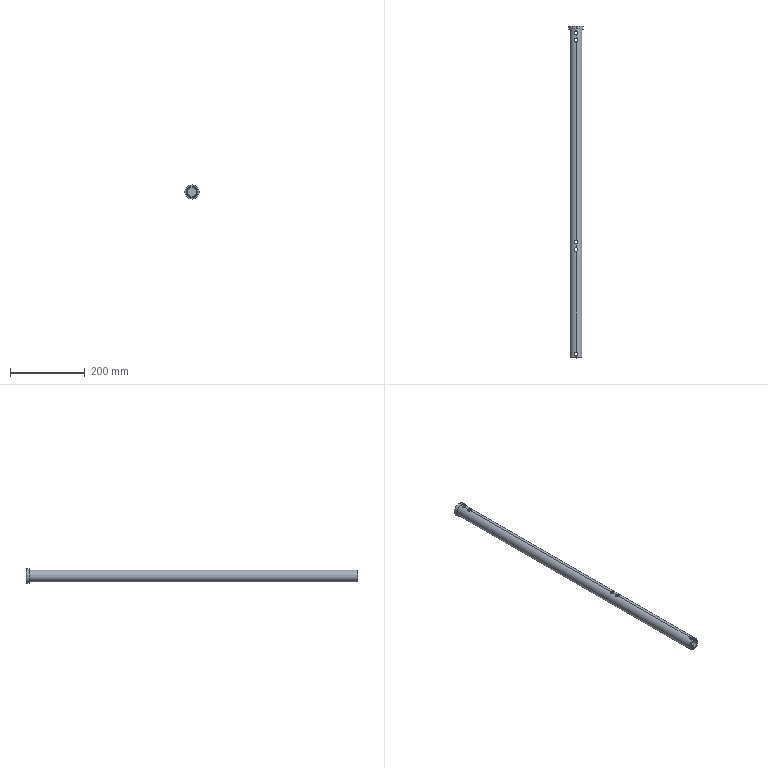Part | SolidWorks | features MirrorStock 1 | 1 solid | 32 faces | box 38 x 888 x 38 mm | volume 315320 mm3 | cylinder 26 | plane 4 | cone 2 | commonest cylinder face diameters 10 x20 24 x2 32 x2 38 x2